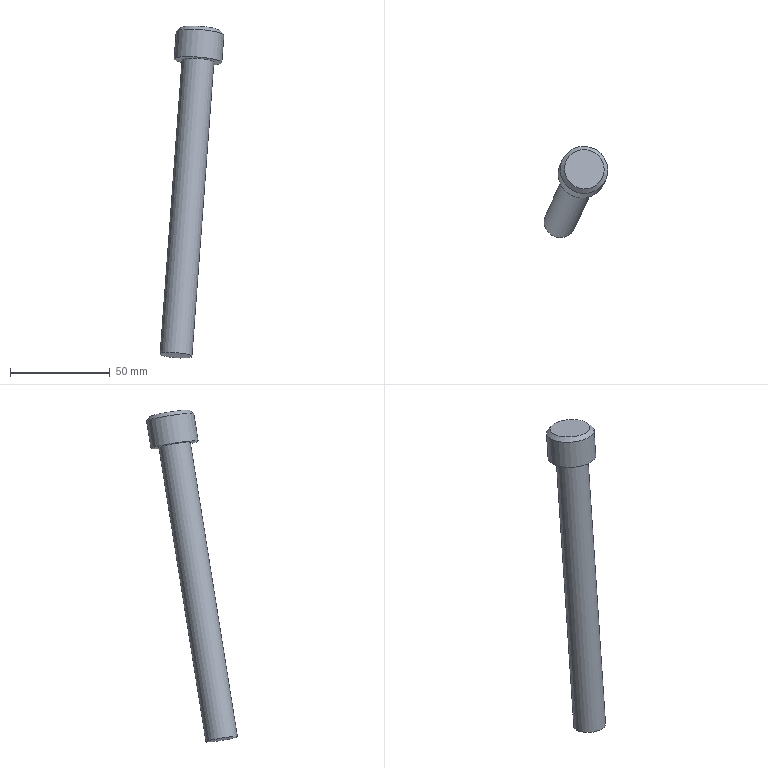Part | NX | features solid 2 | 1 solid | 6 faces | box 31.982 x 45.561 x 166.604 mm | volume 37255 mm3 | plane 3 | cylinder 2 | cone 1 | commonest cylinder face diameters 16 x1 24 x1
STEP:
#1=CARTESIAN_POINT('',(479.76,573.354,245.028));
#2=VERTEX_POINT('',#1);
#3=CARTESIAN_POINT('',(470.697,577.581,245.028));
#4=DIRECTION('',(-0.07339,-0.1574,-0.9848));
#5=DIRECTION('',(0.9063,-0.4226,0.000000001));
#6=AXIS2_PLACEMENT_3D('',#3,#4,#5);
#7=CIRCLE('',#6,10.);
#8=EDGE_CURVE('',#2,#2,#7,.T.);
#9=ORIENTED_EDGE('',*,*,#8,.F.);
#10=EDGE_LOOP('',(#9));
#11=FACE_BOUND('',#10,.T.);
#12=CARTESIAN_POINT('',(470.697,577.581,245.028));
#13=DIRECTION('',(0.07339,0.1574,0.9848));
#14=DIRECTION('',(0.9063,-0.4226,0.000000001));
#15=AXIS2_PLACEMENT_3D('',#12,#13,#14);
#16=PLANE('',#15);
#17=ADVANCED_FACE('',(#11),#16,.T.);
#18=CARTESIAN_POINT('',(462.272,578.443,229.271));
#19=VERTEX_POINT('',#18);
#20=CARTESIAN_POINT('',(469.523,575.063,229.271));
#21=DIRECTION('',(0.07339,0.1574,0.9848));
#22=DIRECTION('',(-0.9063,0.4226,-0.000000001));
#23=AXIS2_PLACEMENT_3D('',#20,#21,#22);
#24=CIRCLE('',#23,8.);
#25=EDGE_CURVE('',#19,#19,#24,.T.);
#26=ORIENTED_EDGE('',*,*,#25,.T.);
#27=EDGE_LOOP('',(#26));
#28=FACE_BOUND('',#27,.T.);
#29=CARTESIAN_POINT('',(480.398,569.991,229.271));
#30=VERTEX_POINT('',#29);
#31=CARTESIAN_POINT('',(469.523,575.063,229.271));
#32=DIRECTION('',(-0.07339,-0.1574,-0.9848));
#33=DIRECTION('',(0.9063,-0.4226,0.000000001));
#34=AXIS2_PLACEMENT_3D('',#31,#32,#33);
#35=CIRCLE('',#34,12.);
#36=EDGE_CURVE('',#30,#30,#35,.T.);
#37=ORIENTED_EDGE('',*,*,#36,.T.);
#38=EDGE_LOOP('',(#37));
#39=FACE_BOUND('',#38,.T.);
#40=CARTESIAN_POINT('',(469.523,575.063,229.271));
#41=DIRECTION('',(-0.07339,-0.1574,-0.9848));
#42=DIRECTION('',(-0.9063,0.4226,-0.000000001));
#43=AXIS2_PLACEMENT_3D('',#40,#41,#42);
#44=PLANE('',#43);
#45=ADVANCED_FACE('',(#28,#39),#44,.T.);
#46=CARTESIAN_POINT('',(481.426,572.194,243.058));
#47=VERTEX_POINT('',#46);
#48=CARTESIAN_POINT('',(470.55,577.266,243.058));
#49=DIRECTION('',(-0.07339,-0.1574,-0.9848));
#50=DIRECTION('',(0.9063,-0.4226,0.000000001));
#51=AXIS2_PLACEMENT_3D('',#48,#49,#50);
#52=CIRCLE('',#51,12.);
#53=EDGE_CURVE('',#47,#47,#52,.F.);
#54=ORIENTED_EDGE('',*,*,#53,.F.);
#55=EDGE_LOOP('',(#54));
#56=FACE_BOUND('',#55,.T.);
#57=ORIENTED_EDGE('',*,*,#36,.F.);
#58=EDGE_LOOP('',(#57));
#59=FACE_BOUND('',#58,.T.);
#60=CARTESIAN_POINT('',(469.523,575.063,229.271));
#61=DIRECTION('',(0.07339,0.1574,0.9848));
#62=DIRECTION('',(0.9063,-0.4226,0.000000001));
#63=AXIS2_PLACEMENT_3D('',#60,#61,#62);
#64=CYLINDRICAL_SURFACE('',#63,12.);
#65=ADVANCED_FACE('',(#56,#59),#64,.T.);
#66=CARTESIAN_POINT('',(451.264,554.837,81.55));
#67=VERTEX_POINT('',#66);
#68=CARTESIAN_POINT('',(458.514,551.456,81.55));
#69=DIRECTION('',(0.07339,0.1574,0.9848));
#70=DIRECTION('',(-0.9063,0.4226,-0.000000001));
#71=AXIS2_PLACEMENT_3D('',#68,#69,#70);
#72=CIRCLE('',#71,8.);
#73=EDGE_CURVE('',#67,#67,#72,.F.);
#74=ORIENTED_EDGE('',*,*,#73,.T.);
#75=EDGE_LOOP('',(#74));
#76=FACE_BOUND('',#75,.T.);
#77=CARTESIAN_POINT('',(458.514,551.456,81.55));
#78=DIRECTION('',(-0.07339,-0.1574,-0.9848));
#79=DIRECTION('',(-0.9063,0.4226,-0.000000001));
#80=AXIS2_PLACEMENT_3D('',#77,#78,#79);
#81=PLANE('',#80);
#82=ADVANCED_FACE('',(#76),#81,.T.);
#83=ORIENTED_EDGE('',*,*,#73,.F.);
#84=EDGE_LOOP('',(#83));
#85=FACE_BOUND('',#84,.T.);
#86=ORIENTED_EDGE('',*,*,#25,.F.);
#87=EDGE_LOOP('',(#86));
#88=FACE_BOUND('',#87,.T.);
#89=CARTESIAN_POINT('',(469.523,575.063,229.271));
#90=DIRECTION('',(-0.07339,-0.1574,-0.9848));
#91=DIRECTION('',(-0.9063,0.4226,-0.000000001));
#92=AXIS2_PLACEMENT_3D('',#89,#90,#91);
#93=CYLINDRICAL_SURFACE('',#92,8.);
#94=ADVANCED_FACE('',(#85,#88),#93,.T.);
#95=ORIENTED_EDGE('',*,*,#8,.T.);
#96=EDGE_LOOP('',(#95));
#97=FACE_BOUND('',#96,.T.);
#98=ORIENTED_EDGE('',*,*,#53,.T.);
#99=EDGE_LOOP('',(#98));
#100=FACE_BOUND('',#99,.T.);
#101=CARTESIAN_POINT('',(470.55,577.266,243.058));
#102=DIRECTION('',(-0.07339,-0.1574,-0.9848));
#103=DIRECTION('',(-0.9063,0.4226,-0.000000001));
#104=AXIS2_PLACEMENT_3D('',#101,#102,#103);
#105=CONICAL_SURFACE('',#104,12.,0.7854);
#106=ADVANCED_FACE('',(#97,#100),#105,.T.);
#107=CLOSED_SHELL('',(#17,#45,#65,#82,#94,#106));
#108=MANIFOLD_SOLID_BREP('',#107);
#109=(LENGTH_UNIT()NAMED_UNIT(*)SI_UNIT(.MILLI.,.METRE.));
#110=UNCERTAINTY_MEASURE_WITH_UNIT(LENGTH_MEASURE(0.00001),#109,'','');
#111=(NAMED_UNIT(*)PLANE_ANGLE_UNIT()SI_UNIT($,.RADIAN.));
#112=(NAMED_UNIT(*)SI_UNIT($,.STERADIAN.)SOLID_ANGLE_UNIT());
#113=(GEOMETRIC_REPRESENTATION_CONTEXT(3)GLOBAL_UNCERTAINTY_ASSIGNED_CONTEXT((#110))GLOBAL_UNIT_ASSIGNED_CONTEXT((#109,#111,#112))REPRESENTATION_CONTEXT('',''));
#114=ADVANCED_BREP_SHAPE_REPRESENTATION('',(#108),#113);